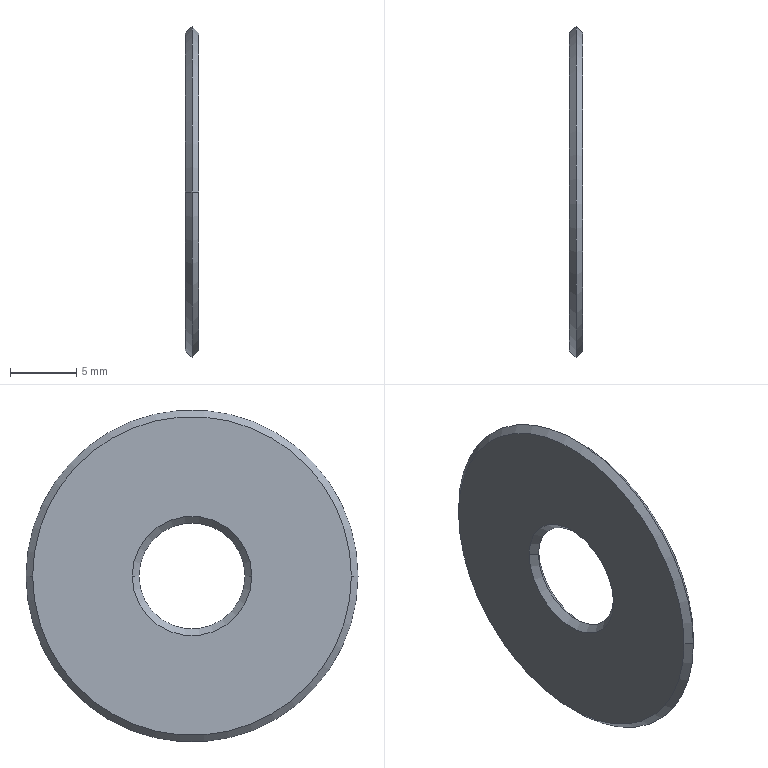Part | STEP file | 0217_006_WSSS25-8-1 | 1 solid | 10 faces | box 1 x 25 x 25 mm | volume 414.69 mm3 | cone 8 | plane 2
STEP:
#1=CARTESIAN_POINT('',(0.,0.,0.));
#2=DIRECTION('',(0.,0.,1.));
#3=DIRECTION('',(1.,0.,0.));
#4=AXIS2_PLACEMENT_3D('',#1,#2,#3);
#5=CARTESIAN_POINT('',(1.,12.,0.));
#6=VERTEX_POINT('',#5);
#7=CARTESIAN_POINT('',(1.,-12.,0.));
#8=VERTEX_POINT('',#7);
#9=CARTESIAN_POINT('',(1.,0.,0.));
#10=DIRECTION('',(1.,0.,0.));
#11=DIRECTION('',(0.,-1.,0.));
#12=AXIS2_PLACEMENT_3D('',#9,#10,#11);
#13=CIRCLE('',#12,12.);
#14=CARTESIAN_POINT('',(0.5,0.,0.));
#15=DIRECTION('',(-1.,0.,0.));
#16=DIRECTION('',(0.,-1.,0.));
#17=AXIS2_PLACEMENT_3D('',#14,#15,#16);
#18=CONICAL_SURFACE('',#17,12.5,0.7854);
#19=CARTESIAN_POINT('',(6.283,-0.5));
#20=DIRECTION('',(-1.,0.));
#21=VECTOR('',#20,1.);
#22=LINE('',#19,#21);
#23=(GEOMETRIC_REPRESENTATION_CONTEXT(2)PARAMETRIC_REPRESENTATION_CONTEXT()REPRESENTATION_CONTEXT('',''));
#24=DEFINITIONAL_REPRESENTATION('',(#22),#23);
#25=PCURVE('',#18,#24);
#26=CARTESIAN_POINT('',(1.,-8.25,0.));
#27=DIRECTION('',(1.,0.,0.));
#28=DIRECTION('',(0.,1.,0.));
#29=AXIS2_PLACEMENT_3D('',#26,#27,#28);
#30=PLANE('',#29);
#31=CARTESIAN_POINT('',(8.25,0.));
#32=DIRECTION('',(-1.,0.));
#33=AXIS2_PLACEMENT_2D('',#31,#32);
#34=CIRCLE('',#33,12.);
#35=(GEOMETRIC_REPRESENTATION_CONTEXT(2)PARAMETRIC_REPRESENTATION_CONTEXT()REPRESENTATION_CONTEXT('',''));
#36=DEFINITIONAL_REPRESENTATION('',(#34),#35);
#37=PCURVE('',#30,#36);
#38=SURFACE_CURVE('',#13,(#25,#37),.PCURVE_S1.);
#39=EDGE_CURVE('',#6,#8,#38,.T.);
#40=ORIENTED_EDGE('',*,*,#39,.F.);
#41=CARTESIAN_POINT('',(0.5,12.5,0.));
#42=VERTEX_POINT('',#41);
#43=CARTESIAN_POINT('',(0.5,12.5,0.));
#44=DIRECTION('',(-0.7071,0.7071,0.));
#45=VECTOR('',#44,1.);
#46=LINE('',#43,#45);
#47=CARTESIAN_POINT('',(3.142,0.));
#48=DIRECTION('',(0.,1.));
#49=VECTOR('',#48,1.);
#50=LINE('',#47,#49);
#51=(GEOMETRIC_REPRESENTATION_CONTEXT(2)PARAMETRIC_REPRESENTATION_CONTEXT()REPRESENTATION_CONTEXT('',''));
#52=DEFINITIONAL_REPRESENTATION('',(#50),#51);
#53=PCURVE('',#18,#52);
#54=CARTESIAN_POINT('',(0.5,0.,0.));
#55=DIRECTION('',(-1.,0.,0.));
#56=DIRECTION('',(0.,-1.,0.));
#57=AXIS2_PLACEMENT_3D('',#54,#55,#56);
#58=CONICAL_SURFACE('',#57,12.5,0.7854);
#59=CARTESIAN_POINT('',(3.142,0.));
#60=DIRECTION('',(0.,1.));
#61=VECTOR('',#60,1.);
#62=LINE('',#59,#61);
#63=(GEOMETRIC_REPRESENTATION_CONTEXT(2)PARAMETRIC_REPRESENTATION_CONTEXT()REPRESENTATION_CONTEXT('',''));
#64=DEFINITIONAL_REPRESENTATION('',(#62),#63);
#65=PCURVE('',#58,#64);
#66=SURFACE_CURVE('',#46,(#53,#65),.PCURVE_S1.);
#67=EDGE_CURVE('',#6,#42,#66,.T.);
#68=ORIENTED_EDGE('',*,*,#67,.T.);
#69=CARTESIAN_POINT('',(0.5,-12.5,0.));
#70=VERTEX_POINT('',#69);
#71=CARTESIAN_POINT('',(0.5,0.,0.));
#72=DIRECTION('',(1.,0.,0.));
#73=DIRECTION('',(0.,-1.,0.));
#74=AXIS2_PLACEMENT_3D('',#71,#72,#73);
#75=CIRCLE('',#74,12.5);
#76=CARTESIAN_POINT('',(6.283,0.));
#77=DIRECTION('',(-1.,0.));
#78=VECTOR('',#77,1.);
#79=LINE('',#76,#78);
#80=(GEOMETRIC_REPRESENTATION_CONTEXT(2)PARAMETRIC_REPRESENTATION_CONTEXT()REPRESENTATION_CONTEXT('',''));
#81=DEFINITIONAL_REPRESENTATION('',(#79),#80);
#82=PCURVE('',#18,#81);
#83=CARTESIAN_POINT('',(0.5,0.,0.));
#84=DIRECTION('',(1.,0.,0.));
#85=DIRECTION('',(0.,1.,0.));
#86=AXIS2_PLACEMENT_3D('',#83,#84,#85);
#87=CONICAL_SURFACE('',#86,12.5,0.7854);
#88=CARTESIAN_POINT('',(-3.142,0.));
#89=DIRECTION('',(1.,0.));
#90=VECTOR('',#89,1.);
#91=LINE('',#88,#90);
#92=(GEOMETRIC_REPRESENTATION_CONTEXT(2)PARAMETRIC_REPRESENTATION_CONTEXT()REPRESENTATION_CONTEXT('',''));
#93=DEFINITIONAL_REPRESENTATION('',(#91),#92);
#94=PCURVE('',#87,#93);
#95=SURFACE_CURVE('',#75,(#82,#94),.PCURVE_S1.);
#96=EDGE_CURVE('',#42,#70,#95,.T.);
#97=ORIENTED_EDGE('',*,*,#96,.T.);
#98=CARTESIAN_POINT('',(0.5,-12.5,0.));
#99=DIRECTION('',(-0.7071,-0.7071,0.));
#100=VECTOR('',#99,1.);
#101=LINE('',#98,#100);
#102=CARTESIAN_POINT('',(0.,0.));
#103=DIRECTION('',(0.,1.));
#104=VECTOR('',#103,1.);
#105=LINE('',#102,#104);
#106=(GEOMETRIC_REPRESENTATION_CONTEXT(2)PARAMETRIC_REPRESENTATION_CONTEXT()REPRESENTATION_CONTEXT('',''));
#107=DEFINITIONAL_REPRESENTATION('',(#105),#106);
#108=PCURVE('',#18,#107);
#109=CARTESIAN_POINT('',(6.283,0.));
#110=DIRECTION('',(0.,1.));
#111=VECTOR('',#110,1.);
#112=LINE('',#109,#111);
#113=(GEOMETRIC_REPRESENTATION_CONTEXT(2)PARAMETRIC_REPRESENTATION_CONTEXT()REPRESENTATION_CONTEXT('',''));
#114=DEFINITIONAL_REPRESENTATION('',(#112),#113);
#115=PCURVE('',#58,#114);
#116=SURFACE_CURVE('',#101,(#108,#115),.PCURVE_S1.);
#117=EDGE_CURVE('',#8,#70,#116,.T.);
#118=ORIENTED_EDGE('',*,*,#117,.F.);
#119=EDGE_LOOP('',(#40,#68,#97,#118));
#120=FACE_BOUND('',#119,.T.);
#121=ADVANCED_FACE('',(#120),#18,.T.);
#122=CARTESIAN_POINT('',(0.5,4.,0.));
#123=VERTEX_POINT('',#122);
#124=CARTESIAN_POINT('',(1.,4.5,0.));
#125=VERTEX_POINT('',#124);
#126=CARTESIAN_POINT('',(1.,4.5,0.));
#127=DIRECTION('',(0.7071,0.7071,0.));
#128=VECTOR('',#127,1.);
#129=LINE('',#126,#128);
#130=CARTESIAN_POINT('',(1.,0.,0.));
#131=DIRECTION('',(1.,0.,0.));
#132=DIRECTION('',(0.,1.,0.));
#133=AXIS2_PLACEMENT_3D('',#130,#131,#132);
#134=CONICAL_SURFACE('',#133,4.5,0.7854);
#135=CARTESIAN_POINT('',(6.283,0.));
#136=DIRECTION('',(0.,1.));
#137=VECTOR('',#136,1.);
#138=LINE('',#135,#137);
#139=(GEOMETRIC_REPRESENTATION_CONTEXT(2)PARAMETRIC_REPRESENTATION_CONTEXT()REPRESENTATION_CONTEXT('',''));
#140=DEFINITIONAL_REPRESENTATION('',(#138),#139);
#141=PCURVE('',#134,#140);
#142=CARTESIAN_POINT('',(1.,0.,0.));
#143=DIRECTION('',(1.,0.,0.));
#144=DIRECTION('',(0.,1.,0.));
#145=AXIS2_PLACEMENT_3D('',#142,#143,#144);
#146=CONICAL_SURFACE('',#145,4.5,0.7854);
#147=CARTESIAN_POINT('',(0.,0.));
#148=DIRECTION('',(0.,1.));
#149=VECTOR('',#148,1.);
#150=LINE('',#147,#149);
#151=(GEOMETRIC_REPRESENTATION_CONTEXT(2)PARAMETRIC_REPRESENTATION_CONTEXT()REPRESENTATION_CONTEXT('',''));
#152=DEFINITIONAL_REPRESENTATION('',(#150),#151);
#153=PCURVE('',#146,#152);
#154=SURFACE_CURVE('',#129,(#141,#153),.PCURVE_S1.);
#155=EDGE_CURVE('',#123,#125,#154,.T.);
#156=ORIENTED_EDGE('',*,*,#155,.T.);
#157=CARTESIAN_POINT('',(1.,-4.5,0.));
#158=VERTEX_POINT('',#157);
#159=CARTESIAN_POINT('',(1.,0.,0.));
#160=DIRECTION('',(-1.,0.,0.));
#161=DIRECTION('',(0.,1.,0.));
#162=AXIS2_PLACEMENT_3D('',#159,#160,#161);
#163=CIRCLE('',#162,4.5);
#164=CARTESIAN_POINT('',(6.283,0.));
#165=DIRECTION('',(-1.,0.));
#166=VECTOR('',#165,1.);
#167=LINE('',#164,#166);
#168=(GEOMETRIC_REPRESENTATION_CONTEXT(2)PARAMETRIC_REPRESENTATION_CONTEXT()REPRESENTATION_CONTEXT('',''));
#169=DEFINITIONAL_REPRESENTATION('',(#167),#168);
#170=PCURVE('',#134,#169);
#171=CARTESIAN_POINT('',(12.75,0.));
#172=CARTESIAN_POINT('',(12.75,-7.794));
#173=CARTESIAN_POINT('',(6.,-3.897));
#174=CARTESIAN_POINT('',(-0.75,0.));
#175=CARTESIAN_POINT('',(6.,3.897));
#176=CARTESIAN_POINT('',(12.75,7.794));
#177=CARTESIAN_POINT('',(12.75,0.));
#178=(BOUNDED_CURVE()B_SPLINE_CURVE(2,(#171,#172,#173,#174,#175,#176,#177),.UNSPECIFIED.,.T.,.F.)B_SPLINE_CURVE_WITH_KNOTS((1,2,2,2,2,1),(-2.094,0.,2.094,4.189,6.283,8.378),.UNSPECIFIED.)CURVE()GEOMETRIC_REPRESENTATION_ITEM()RATIONAL_B_SPLINE_CURVE((1.,0.5,1.,0.5,1.,0.5,1.))REPRESENTATION_ITEM(''));
#179=(GEOMETRIC_REPRESENTATION_CONTEXT(2)PARAMETRIC_REPRESENTATION_CONTEXT()REPRESENTATION_CONTEXT('',''));
#180=DEFINITIONAL_REPRESENTATION('',(#178),#179);
#181=PCURVE('',#30,#180);
#182=SURFACE_CURVE('',#163,(#170,#181),.PCURVE_S1.);
#183=EDGE_CURVE('',#125,#158,#182,.T.);
#184=ORIENTED_EDGE('',*,*,#183,.T.);
#185=CARTESIAN_POINT('',(0.5,-4.,0.));
#186=VERTEX_POINT('',#185);
#187=CARTESIAN_POINT('',(1.,-4.5,0.));
#188=DIRECTION('',(0.7071,-0.7071,0.));
#189=VECTOR('',#188,1.);
#190=LINE('',#187,#189);
#191=CARTESIAN_POINT('',(3.142,0.));
#192=DIRECTION('',(0.,1.));
#193=VECTOR('',#192,1.);
#194=LINE('',#191,#193);
#195=(GEOMETRIC_REPRESENTATION_CONTEXT(2)PARAMETRIC_REPRESENTATION_CONTEXT()REPRESENTATION_CONTEXT('',''));
#196=DEFINITIONAL_REPRESENTATION('',(#194),#195);
#197=PCURVE('',#134,#196);
#198=CARTESIAN_POINT('',(3.142,0.));
#199=DIRECTION('',(0.,1.));
#200=VECTOR('',#199,1.);
#201=LINE('',#198,#200);
#202=(GEOMETRIC_REPRESENTATION_CONTEXT(2)PARAMETRIC_REPRESENTATION_CONTEXT()REPRESENTATION_CONTEXT('',''));
#203=DEFINITIONAL_REPRESENTATION('',(#201),#202);
#204=PCURVE('',#146,#203);
#205=SURFACE_CURVE('',#190,(#197,#204),.PCURVE_S1.);
#206=EDGE_CURVE('',#186,#158,#205,.T.);
#207=ORIENTED_EDGE('',*,*,#206,.F.);
#208=CARTESIAN_POINT('',(0.5,0.,0.));
#209=DIRECTION('',(1.,0.,0.));
#210=DIRECTION('',(0.,-1.,0.));
#211=AXIS2_PLACEMENT_3D('',#208,#209,#210);
#212=CIRCLE('',#211,4.);
#213=CARTESIAN_POINT('',(3.142,-0.5));
#214=DIRECTION('',(1.,0.));
#215=VECTOR('',#214,1.);
#216=LINE('',#213,#215);
#217=(GEOMETRIC_REPRESENTATION_CONTEXT(2)PARAMETRIC_REPRESENTATION_CONTEXT()REPRESENTATION_CONTEXT('',''));
#218=DEFINITIONAL_REPRESENTATION('',(#216),#217);
#219=PCURVE('',#134,#218);
#220=CARTESIAN_POINT('',(0.,0.,0.));
#221=DIRECTION('',(-1.,0.,0.));
#222=DIRECTION('',(0.,-1.,0.));
#223=AXIS2_PLACEMENT_3D('',#220,#221,#222);
#224=CONICAL_SURFACE('',#223,4.5,0.7854);
#225=CARTESIAN_POINT('',(6.283,-0.5));
#226=DIRECTION('',(-1.,0.));
#227=VECTOR('',#226,1.);
#228=LINE('',#225,#227);
#229=(GEOMETRIC_REPRESENTATION_CONTEXT(2)PARAMETRIC_REPRESENTATION_CONTEXT()REPRESENTATION_CONTEXT('',''));
#230=DEFINITIONAL_REPRESENTATION('',(#228),#229);
#231=PCURVE('',#224,#230);
#232=SURFACE_CURVE('',#212,(#219,#231),.PCURVE_S1.);
#233=EDGE_CURVE('',#186,#123,#232,.T.);
#234=ORIENTED_EDGE('',*,*,#233,.T.);
#235=EDGE_LOOP('',(#156,#184,#207,#234));
#236=FACE_BOUND('',#235,.F.);
#237=ADVANCED_FACE('',(#236),#134,.F.);
#238=CARTESIAN_POINT('',(0.,12.,0.));
#239=VERTEX_POINT('',#238);
#240=CARTESIAN_POINT('',(0.,-12.,0.));
#241=VERTEX_POINT('',#240);
#242=CARTESIAN_POINT('',(0.,0.,0.));
#243=DIRECTION('',(1.,0.,0.));
#244=DIRECTION('',(0.,1.,0.));
#245=AXIS2_PLACEMENT_3D('',#242,#243,#244);
#246=CIRCLE('',#245,12.);
#247=CARTESIAN_POINT('',(0.,-0.5));
#248=DIRECTION('',(1.,0.));
#249=VECTOR('',#248,1.);
#250=LINE('',#247,#249);
#251=(GEOMETRIC_REPRESENTATION_CONTEXT(2)PARAMETRIC_REPRESENTATION_CONTEXT()REPRESENTATION_CONTEXT('',''));
#252=DEFINITIONAL_REPRESENTATION('',(#250),#251);
#253=PCURVE('',#87,#252);
#254=CARTESIAN_POINT('',(0.,-8.25,0.));
#255=DIRECTION('',(-1.,0.,0.));
#256=DIRECTION('',(0.,-1.,0.));
#257=AXIS2_PLACEMENT_3D('',#254,#255,#256);
#258=PLANE('',#257);
#259=CARTESIAN_POINT('',(-20.25,0.));
#260=CARTESIAN_POINT('',(-20.25,20.785));
#261=CARTESIAN_POINT('',(-2.25,10.392));
#262=CARTESIAN_POINT('',(15.75,0.));
#263=CARTESIAN_POINT('',(-2.25,-10.392));
#264=CARTESIAN_POINT('',(-20.25,-20.785));
#265=CARTESIAN_POINT('',(-20.25,0.));
#266=(BOUNDED_CURVE()B_SPLINE_CURVE(2,(#259,#260,#261,#262,#263,#264,#265),.UNSPECIFIED.,.T.,.F.)B_SPLINE_CURVE_WITH_KNOTS((1,2,2,2,2,1),(-2.094,0.,2.094,4.189,6.283,8.378),.UNSPECIFIED.)CURVE()GEOMETRIC_REPRESENTATION_ITEM()RATIONAL_B_SPLINE_CURVE((1.,0.5,1.,0.5,1.,0.5,1.))REPRESENTATION_ITEM(''));
#267=(GEOMETRIC_REPRESENTATION_CONTEXT(2)PARAMETRIC_REPRESENTATION_CONTEXT()REPRESENTATION_CONTEXT('',''));
#268=DEFINITIONAL_REPRESENTATION('',(#266),#267);
#269=PCURVE('',#258,#268);
#270=SURFACE_CURVE('',#246,(#253,#269),.PCURVE_S1.);
#271=EDGE_CURVE('',#239,#241,#270,.T.);
#272=ORIENTED_EDGE('',*,*,#271,.T.);
#273=CARTESIAN_POINT('',(0.5,-12.5,0.));
#274=DIRECTION('',(0.7071,-0.7071,0.));
#275=VECTOR('',#274,1.);
#276=LINE('',#273,#275);
#277=CARTESIAN_POINT('',(3.142,0.));
#278=DIRECTION('',(0.,1.));
#279=VECTOR('',#278,1.);
#280=LINE('',#277,#279);
#281=(GEOMETRIC_REPRESENTATION_CONTEXT(2)PARAMETRIC_REPRESENTATION_CONTEXT()REPRESENTATION_CONTEXT('',''));
#282=DEFINITIONAL_REPRESENTATION('',(#280),#281);
#283=PCURVE('',#87,#282);
#284=CARTESIAN_POINT('',(0.5,0.,0.));
#285=DIRECTION('',(1.,0.,0.));
#286=DIRECTION('',(0.,1.,0.));
#287=AXIS2_PLACEMENT_3D('',#284,#285,#286);
#288=CONICAL_SURFACE('',#287,12.5,0.7854);
#289=CARTESIAN_POINT('',(3.142,0.));
#290=DIRECTION('',(0.,1.));
#291=VECTOR('',#290,1.);
#292=LINE('',#289,#291);
#293=(GEOMETRIC_REPRESENTATION_CONTEXT(2)PARAMETRIC_REPRESENTATION_CONTEXT()REPRESENTATION_CONTEXT('',''));
#294=DEFINITIONAL_REPRESENTATION('',(#292),#293);
#295=PCURVE('',#288,#294);
#296=SURFACE_CURVE('',#276,(#283,#295),.PCURVE_S1.);
#297=EDGE_CURVE('',#241,#70,#296,.T.);
#298=ORIENTED_EDGE('',*,*,#297,.T.);
#299=ORIENTED_EDGE('',*,*,#96,.F.);
#300=CARTESIAN_POINT('',(0.5,12.5,0.));
#301=DIRECTION('',(0.7071,0.7071,0.));
#302=VECTOR('',#301,1.);
#303=LINE('',#300,#302);
#304=CARTESIAN_POINT('',(0.,0.));
#305=DIRECTION('',(0.,1.));
#306=VECTOR('',#305,1.);
#307=LINE('',#304,#306);
#308=(GEOMETRIC_REPRESENTATION_CONTEXT(2)PARAMETRIC_REPRESENTATION_CONTEXT()REPRESENTATION_CONTEXT('',''));
#309=DEFINITIONAL_REPRESENTATION('',(#307),#308);
#310=PCURVE('',#87,#309);
#311=CARTESIAN_POINT('',(6.283,0.));
#312=DIRECTION('',(0.,1.));
#313=VECTOR('',#312,1.);
#314=LINE('',#311,#313);
#315=(GEOMETRIC_REPRESENTATION_CONTEXT(2)PARAMETRIC_REPRESENTATION_CONTEXT()REPRESENTATION_CONTEXT('',''));
#316=DEFINITIONAL_REPRESENTATION('',(#314),#315);
#317=PCURVE('',#288,#316);
#318=SURFACE_CURVE('',#303,(#310,#317),.PCURVE_S1.);
#319=EDGE_CURVE('',#239,#42,#318,.T.);
#320=ORIENTED_EDGE('',*,*,#319,.F.);
#321=EDGE_LOOP('',(#272,#298,#299,#320));
#322=FACE_BOUND('',#321,.T.);
#323=ADVANCED_FACE('',(#322),#87,.T.);
#324=CARTESIAN_POINT('',(0.,-4.5,0.));
#325=VERTEX_POINT('',#324);
#326=CARTESIAN_POINT('',(0.,-4.5,0.));
#327=DIRECTION('',(-0.7071,-0.7071,0.));
#328=VECTOR('',#327,1.);
#329=LINE('',#326,#328);
#330=CARTESIAN_POINT('',(6.283,0.));
#331=DIRECTION('',(0.,1.));
#332=VECTOR('',#331,1.);
#333=LINE('',#330,#332);
#334=(GEOMETRIC_REPRESENTATION_CONTEXT(2)PARAMETRIC_REPRESENTATION_CONTEXT()REPRESENTATION_CONTEXT('',''));
#335=DEFINITIONAL_REPRESENTATION('',(#333),#334);
#336=PCURVE('',#224,#335);
#337=CARTESIAN_POINT('',(0.,0.,0.));
#338=DIRECTION('',(-1.,0.,0.));
#339=DIRECTION('',(0.,-1.,0.));
#340=AXIS2_PLACEMENT_3D('',#337,#338,#339);
#341=CONICAL_SURFACE('',#340,4.5,0.7854);
#342=CARTESIAN_POINT('',(0.,0.));
#343=DIRECTION('',(0.,1.));
#344=VECTOR('',#343,1.);
#345=LINE('',#342,#344);
#346=(GEOMETRIC_REPRESENTATION_CONTEXT(2)PARAMETRIC_REPRESENTATION_CONTEXT()REPRESENTATION_CONTEXT('',''));
#347=DEFINITIONAL_REPRESENTATION('',(#345),#346);
#348=PCURVE('',#341,#347);
#349=SURFACE_CURVE('',#329,(#336,#348),.PCURVE_S1.);
#350=EDGE_CURVE('',#186,#325,#349,.T.);
#351=ORIENTED_EDGE('',*,*,#350,.T.);
#352=CARTESIAN_POINT('',(0.,4.5,0.));
#353=VERTEX_POINT('',#352);
#354=CARTESIAN_POINT('',(0.,0.,0.));
#355=DIRECTION('',(1.,0.,0.));
#356=DIRECTION('',(0.,-1.,0.));
#357=AXIS2_PLACEMENT_3D('',#354,#355,#356);
#358=CIRCLE('',#357,4.5);
#359=CARTESIAN_POINT('',(6.283,0.));
#360=DIRECTION('',(-1.,0.));
#361=VECTOR('',#360,1.);
#362=LINE('',#359,#361);
#363=(GEOMETRIC_REPRESENTATION_CONTEXT(2)PARAMETRIC_REPRESENTATION_CONTEXT()REPRESENTATION_CONTEXT('',''));
#364=DEFINITIONAL_REPRESENTATION('',(#362),#363);
#365=PCURVE('',#224,#364);
#366=CARTESIAN_POINT('',(-3.75,0.));
#367=CARTESIAN_POINT('',(-3.75,-7.794));
#368=CARTESIAN_POINT('',(-10.5,-3.897));
#369=CARTESIAN_POINT('',(-17.25,0.));
#370=CARTESIAN_POINT('',(-10.5,3.897));
#371=CARTESIAN_POINT('',(-3.75,7.794));
#372=CARTESIAN_POINT('',(-3.75,0.));
#373=(BOUNDED_CURVE()B_SPLINE_CURVE(2,(#366,#367,#368,#369,#370,#371,#372),.UNSPECIFIED.,.T.,.F.)B_SPLINE_CURVE_WITH_KNOTS((1,2,2,2,2,1),(-2.094,0.,2.094,4.189,6.283,8.378),.UNSPECIFIED.)CURVE()GEOMETRIC_REPRESENTATION_ITEM()RATIONAL_B_SPLINE_CURVE((1.,0.5,1.,0.5,1.,0.5,1.))REPRESENTATION_ITEM(''));
#374=(GEOMETRIC_REPRESENTATION_CONTEXT(2)PARAMETRIC_REPRESENTATION_CONTEXT()REPRESENTATION_CONTEXT('',''));
#375=DEFINITIONAL_REPRESENTATION('',(#373),#374);
#376=PCURVE('',#258,#375);
#377=SURFACE_CURVE('',#358,(#365,#376),.PCURVE_S1.);
#378=EDGE_CURVE('',#325,#353,#377,.T.);
#379=ORIENTED_EDGE('',*,*,#378,.T.);
#380=CARTESIAN_POINT('',(0.,4.5,0.));
#381=DIRECTION('',(-0.7071,0.7071,0.));
#382=VECTOR('',#381,1.);
#383=LINE('',#380,#382);
#384=CARTESIAN_POINT('',(3.142,0.));
#385=DIRECTION('',(0.,1.));
#386=VECTOR('',#385,1.);
#387=LINE('',#384,#386);
#388=(GEOMETRIC_REPRESENTATION_CONTEXT(2)PARAMETRIC_REPRESENTATION_CONTEXT()REPRESENTATION_CONTEXT('',''));
#389=DEFINITIONAL_REPRESENTATION('',(#387),#388);
#390=PCURVE('',#224,#389);
#391=CARTESIAN_POINT('',(3.142,0.));
#392=DIRECTION('',(0.,1.));
#393=VECTOR('',#392,1.);
#394=LINE('',#391,#393);
#395=(GEOMETRIC_REPRESENTATION_CONTEXT(2)PARAMETRIC_REPRESENTATION_CONTEXT()REPRESENTATION_CONTEXT('',''));
#396=DEFINITIONAL_REPRESENTATION('',(#394),#395);
#397=PCURVE('',#341,#396);
#398=SURFACE_CURVE('',#383,(#390,#397),.PCURVE_S1.);
#399=EDGE_CURVE('',#123,#353,#398,.T.);
#400=ORIENTED_EDGE('',*,*,#399,.F.);
#401=ORIENTED_EDGE('',*,*,#233,.F.);
#402=EDGE_LOOP('',(#351,#379,#400,#401));
#403=FACE_BOUND('',#402,.F.);
#404=ADVANCED_FACE('',(#403),#224,.F.);
#405=CARTESIAN_POINT('',(1.,0.,0.));
#406=DIRECTION('',(1.,0.,0.));
#407=DIRECTION('',(0.,-1.,0.));
#408=AXIS2_PLACEMENT_3D('',#405,#406,#407);
#409=CIRCLE('',#408,12.);
#410=CARTESIAN_POINT('',(8.25,0.));
#411=DIRECTION('',(-1.,0.));
#412=AXIS2_PLACEMENT_2D('',#410,#411);
#413=CIRCLE('',#412,12.);
#414=(GEOMETRIC_REPRESENTATION_CONTEXT(2)PARAMETRIC_REPRESENTATION_CONTEXT()REPRESENTATION_CONTEXT('',''));
#415=DEFINITIONAL_REPRESENTATION('',(#413),#414);
#416=PCURVE('',#30,#415);
#417=CARTESIAN_POINT('',(6.283,-0.5));
#418=DIRECTION('',(-1.,0.));
#419=VECTOR('',#418,1.);
#420=LINE('',#417,#419);
#421=(GEOMETRIC_REPRESENTATION_CONTEXT(2)PARAMETRIC_REPRESENTATION_CONTEXT()REPRESENTATION_CONTEXT('',''));
#422=DEFINITIONAL_REPRESENTATION('',(#420),#421);
#423=PCURVE('',#58,#422);
#424=SURFACE_CURVE('',#409,(#416,#423),.PCURVE_S1.);
#425=EDGE_CURVE('',#8,#6,#424,.T.);
#426=ORIENTED_EDGE('',*,*,#425,.T.);
#427=ORIENTED_EDGE('',*,*,#39,.T.);
#428=EDGE_LOOP('',(#426,#427));
#429=FACE_BOUND('',#428,.T.);
#430=ORIENTED_EDGE('',*,*,#183,.T.);
#431=CARTESIAN_POINT('',(1.,0.,0.));
#432=DIRECTION('',(-1.,0.,0.));
#433=DIRECTION('',(0.,1.,0.));
#434=AXIS2_PLACEMENT_3D('',#431,#432,#433);
#435=CIRCLE('',#434,4.5);
#436=CARTESIAN_POINT('',(12.75,0.));
#437=CARTESIAN_POINT('',(12.75,-7.794));
#438=CARTESIAN_POINT('',(6.,-3.897));
#439=CARTESIAN_POINT('',(-0.75,0.));
#440=CARTESIAN_POINT('',(6.,3.897));
#441=CARTESIAN_POINT('',(12.75,7.794));
#442=CARTESIAN_POINT('',(12.75,0.));
#443=(BOUNDED_CURVE()B_SPLINE_CURVE(2,(#436,#437,#438,#439,#440,#441,#442),.UNSPECIFIED.,.T.,.F.)B_SPLINE_CURVE_WITH_KNOTS((1,2,2,2,2,1),(-2.094,0.,2.094,4.189,6.283,8.378),.UNSPECIFIED.)CURVE()GEOMETRIC_REPRESENTATION_ITEM()RATIONAL_B_SPLINE_CURVE((1.,0.5,1.,0.5,1.,0.5,1.))REPRESENTATION_ITEM(''));
#444=(GEOMETRIC_REPRESENTATION_CONTEXT(2)PARAMETRIC_REPRESENTATION_CONTEXT()REPRESENTATION_CONTEXT('',''));
#445=DEFINITIONAL_REPRESENTATION('',(#443),#444);
#446=PCURVE('',#30,#445);
#447=CARTESIAN_POINT('',(6.283,0.));
#448=DIRECTION('',(-1.,0.));
#449=VECTOR('',#448,1.);
#450=LINE('',#447,#449);
#451=(GEOMETRIC_REPRESENTATION_CONTEXT(2)PARAMETRIC_REPRESENTATION_CONTEXT()REPRESENTATION_CONTEXT('',''));
#452=DEFINITIONAL_REPRESENTATION('',(#450),#451);
#453=PCURVE('',#146,#452);
#454=SURFACE_CURVE('',#435,(#446,#453),.PCURVE_S1.);
#455=EDGE_CURVE('',#158,#125,#454,.T.);
#456=ORIENTED_EDGE('',*,*,#455,.T.);
#457=EDGE_LOOP('',(#430,#456));
#458=FACE_BOUND('',#457,.T.);
#459=ADVANCED_FACE('',(#429,#458),#30,.T.);
#460=ORIENTED_EDGE('',*,*,#67,.F.);
#461=ORIENTED_EDGE('',*,*,#425,.F.);
#462=ORIENTED_EDGE('',*,*,#117,.T.);
#463=CARTESIAN_POINT('',(0.5,0.,0.));
#464=DIRECTION('',(1.,0.,0.));
#465=DIRECTION('',(0.,-1.,0.));
#466=AXIS2_PLACEMENT_3D('',#463,#464,#465);
#467=CIRCLE('',#466,12.5);
#468=CARTESIAN_POINT('',(6.283,0.));
#469=DIRECTION('',(-1.,0.));
#470=VECTOR('',#469,1.);
#471=LINE('',#468,#470);
#472=(GEOMETRIC_REPRESENTATION_CONTEXT(2)PARAMETRIC_REPRESENTATION_CONTEXT()REPRESENTATION_CONTEXT('',''));
#473=DEFINITIONAL_REPRESENTATION('',(#471),#472);
#474=PCURVE('',#58,#473);
#475=CARTESIAN_POINT('',(3.142,0.));
#476=DIRECTION('',(1.,0.));
#477=VECTOR('',#476,1.);
#478=LINE('',#475,#477);
#479=(GEOMETRIC_REPRESENTATION_CONTEXT(2)PARAMETRIC_REPRESENTATION_CONTEXT()REPRESENTATION_CONTEXT('',''));
#480=DEFINITIONAL_REPRESENTATION('',(#478),#479);
#481=PCURVE('',#288,#480);
#482=SURFACE_CURVE('',#467,(#474,#481),.PCURVE_S1.);
#483=EDGE_CURVE('',#70,#42,#482,.T.);
#484=ORIENTED_EDGE('',*,*,#483,.T.);
#485=EDGE_LOOP('',(#460,#461,#462,#484));
#486=FACE_BOUND('',#485,.T.);
#487=ADVANCED_FACE('',(#486),#58,.T.);
#488=ORIENTED_EDGE('',*,*,#455,.T.);
#489=ORIENTED_EDGE('',*,*,#155,.F.);
#490=CARTESIAN_POINT('',(0.5,0.,0.));
#491=DIRECTION('',(1.,0.,0.));
#492=DIRECTION('',(0.,-1.,0.));
#493=AXIS2_PLACEMENT_3D('',#490,#491,#492);
#494=CIRCLE('',#493,4.);
#495=CARTESIAN_POINT('',(-3.142,-0.5));
#496=DIRECTION('',(1.,0.));
#497=VECTOR('',#496,1.);
#498=LINE('',#495,#497);
#499=(GEOMETRIC_REPRESENTATION_CONTEXT(2)PARAMETRIC_REPRESENTATION_CONTEXT()REPRESENTATION_CONTEXT('',''));
#500=DEFINITIONAL_REPRESENTATION('',(#498),#499);
#501=PCURVE('',#146,#500);
#502=CARTESIAN_POINT('',(6.283,-0.5));
#503=DIRECTION('',(-1.,0.));
#504=VECTOR('',#503,1.);
#505=LINE('',#502,#504);
#506=(GEOMETRIC_REPRESENTATION_CONTEXT(2)PARAMETRIC_REPRESENTATION_CONTEXT()REPRESENTATION_CONTEXT('',''));
#507=DEFINITIONAL_REPRESENTATION('',(#505),#506);
#508=PCURVE('',#341,#507);
#509=SURFACE_CURVE('',#494,(#501,#508),.PCURVE_S1.);
#510=EDGE_CURVE('',#123,#186,#509,.T.);
#511=ORIENTED_EDGE('',*,*,#510,.T.);
#512=ORIENTED_EDGE('',*,*,#206,.T.);
#513=EDGE_LOOP('',(#488,#489,#511,#512));
#514=FACE_BOUND('',#513,.F.);
#515=ADVANCED_FACE('',(#514),#146,.F.);
#516=ORIENTED_EDGE('',*,*,#297,.F.);
#517=CARTESIAN_POINT('',(0.,0.,0.));
#518=DIRECTION('',(1.,0.,0.));
#519=DIRECTION('',(0.,1.,0.));
#520=AXIS2_PLACEMENT_3D('',#517,#518,#519);
#521=CIRCLE('',#520,12.);
#522=CARTESIAN_POINT('',(0.,-0.5));
#523=DIRECTION('',(1.,0.));
#524=VECTOR('',#523,1.);
#525=LINE('',#522,#524);
#526=(GEOMETRIC_REPRESENTATION_CONTEXT(2)PARAMETRIC_REPRESENTATION_CONTEXT()REPRESENTATION_CONTEXT('',''));
#527=DEFINITIONAL_REPRESENTATION('',(#525),#526);
#528=PCURVE('',#288,#527);
#529=CARTESIAN_POINT('',(-20.25,0.));
#530=CARTESIAN_POINT('',(-20.25,20.785));
#531=CARTESIAN_POINT('',(-2.25,10.392));
#532=CARTESIAN_POINT('',(15.75,0.));
#533=CARTESIAN_POINT('',(-2.25,-10.392));
#534=CARTESIAN_POINT('',(-20.25,-20.785));
#535=CARTESIAN_POINT('',(-20.25,0.));
#536=(BOUNDED_CURVE()B_SPLINE_CURVE(2,(#529,#530,#531,#532,#533,#534,#535),.UNSPECIFIED.,.T.,.F.)B_SPLINE_CURVE_WITH_KNOTS((1,2,2,2,2,1),(-2.094,0.,2.094,4.189,6.283,8.378),.UNSPECIFIED.)CURVE()GEOMETRIC_REPRESENTATION_ITEM()RATIONAL_B_SPLINE_CURVE((1.,0.5,1.,0.5,1.,0.5,1.))REPRESENTATION_ITEM(''));
#537=(GEOMETRIC_REPRESENTATION_CONTEXT(2)PARAMETRIC_REPRESENTATION_CONTEXT()REPRESENTATION_CONTEXT('',''));
#538=DEFINITIONAL_REPRESENTATION('',(#536),#537);
#539=PCURVE('',#258,#538);
#540=SURFACE_CURVE('',#521,(#528,#539),.PCURVE_S1.);
#541=EDGE_CURVE('',#241,#239,#540,.T.);
#542=ORIENTED_EDGE('',*,*,#541,.T.);
#543=ORIENTED_EDGE('',*,*,#319,.T.);
#544=ORIENTED_EDGE('',*,*,#483,.F.);
#545=EDGE_LOOP('',(#516,#542,#543,#544));
#546=FACE_BOUND('',#545,.T.);
#547=ADVANCED_FACE('',(#546),#288,.T.);
#548=CARTESIAN_POINT('',(0.,0.,0.));
#549=DIRECTION('',(1.,0.,0.));
#550=DIRECTION('',(0.,-1.,0.));
#551=AXIS2_PLACEMENT_3D('',#548,#549,#550);
#552=CIRCLE('',#551,4.5);
#553=CARTESIAN_POINT('',(6.283,0.));
#554=DIRECTION('',(-1.,0.));
#555=VECTOR('',#554,1.);
#556=LINE('',#553,#555);
#557=(GEOMETRIC_REPRESENTATION_CONTEXT(2)PARAMETRIC_REPRESENTATION_CONTEXT()REPRESENTATION_CONTEXT('',''));
#558=DEFINITIONAL_REPRESENTATION('',(#556),#557);
#559=PCURVE('',#341,#558);
#560=CARTESIAN_POINT('',(-3.75,0.));
#561=CARTESIAN_POINT('',(-3.75,-7.794));
#562=CARTESIAN_POINT('',(-10.5,-3.897));
#563=CARTESIAN_POINT('',(-17.25,0.));
#564=CARTESIAN_POINT('',(-10.5,3.897));
#565=CARTESIAN_POINT('',(-3.75,7.794));
#566=CARTESIAN_POINT('',(-3.75,0.));
#567=(BOUNDED_CURVE()B_SPLINE_CURVE(2,(#560,#561,#562,#563,#564,#565,#566),.UNSPECIFIED.,.T.,.F.)B_SPLINE_CURVE_WITH_KNOTS((1,2,2,2,2,1),(-2.094,0.,2.094,4.189,6.283,8.378),.UNSPECIFIED.)CURVE()GEOMETRIC_REPRESENTATION_ITEM()RATIONAL_B_SPLINE_CURVE((1.,0.5,1.,0.5,1.,0.5,1.))REPRESENTATION_ITEM(''));
#568=(GEOMETRIC_REPRESENTATION_CONTEXT(2)PARAMETRIC_REPRESENTATION_CONTEXT()REPRESENTATION_CONTEXT('',''));
#569=DEFINITIONAL_REPRESENTATION('',(#567),#568);
#570=PCURVE('',#258,#569);
#571=SURFACE_CURVE('',#552,(#559,#570),.PCURVE_S1.);
#572=EDGE_CURVE('',#353,#325,#571,.T.);
#573=ORIENTED_EDGE('',*,*,#572,.T.);
#574=ORIENTED_EDGE('',*,*,#350,.F.);
#575=ORIENTED_EDGE('',*,*,#510,.F.);
#576=ORIENTED_EDGE('',*,*,#399,.T.);
#577=EDGE_LOOP('',(#573,#574,#575,#576));
#578=FACE_BOUND('',#577,.F.);
#579=ADVANCED_FACE('',(#578),#341,.F.);
#580=ORIENTED_EDGE('',*,*,#378,.T.);
#581=ORIENTED_EDGE('',*,*,#572,.T.);
#582=EDGE_LOOP('',(#580,#581));
#583=FACE_BOUND('',#582,.T.);
#584=ORIENTED_EDGE('',*,*,#271,.F.);
#585=ORIENTED_EDGE('',*,*,#541,.F.);
#586=EDGE_LOOP('',(#584,#585));
#587=FACE_BOUND('',#586,.T.);
#588=ADVANCED_FACE('',(#583,#587),#258,.T.);
#589=CLOSED_SHELL('',(#121,#237,#323,#404,#459,#487,#515,#547,#579,#588));
#590=MANIFOLD_SOLID_BREP('',#589);
#591=(LENGTH_UNIT()NAMED_UNIT(*)SI_UNIT(.MILLI.,.METRE.));
#592=UNCERTAINTY_MEASURE_WITH_UNIT(LENGTH_MEASURE(0.0000001),#591,'','');
#593=(NAMED_UNIT(*)PLANE_ANGLE_UNIT()SI_UNIT($,.RADIAN.));
#594=(NAMED_UNIT(*)SI_UNIT($,.STERADIAN.)SOLID_ANGLE_UNIT());
#595=(GEOMETRIC_REPRESENTATION_CONTEXT(3)GLOBAL_UNCERTAINTY_ASSIGNED_CONTEXT((#592))GLOBAL_UNIT_ASSIGNED_CONTEXT((#591,#593,#594))REPRESENTATION_CONTEXT('',''));
#596=ADVANCED_BREP_SHAPE_REPRESENTATION('',(#4,#590),#595);